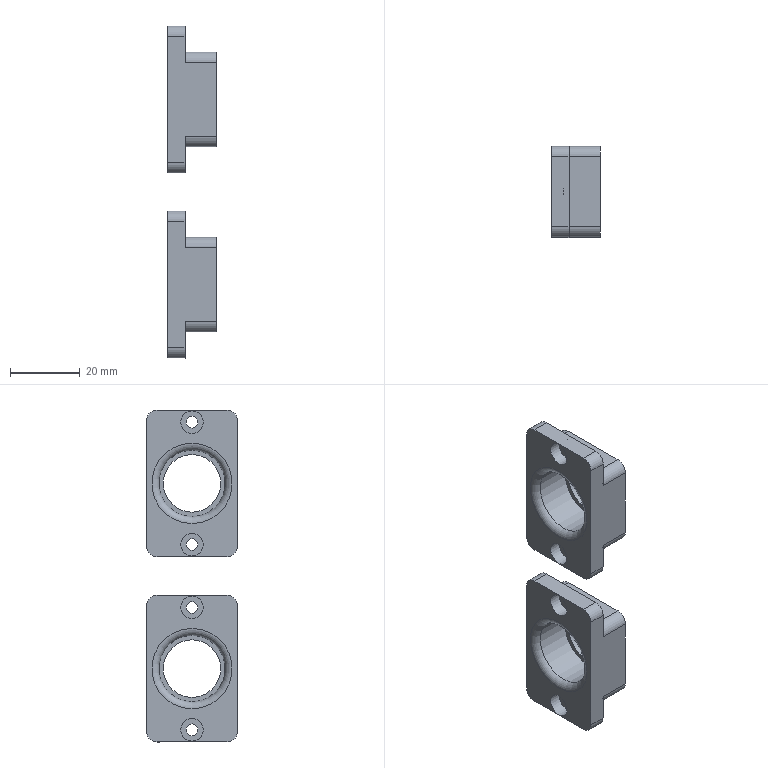CAM job | NX | 3+2 milling, drilling | part box 14 x 26 x 95 mm | stock box 20 x 31 x 100 mm
Tools:
number,name,description,diameter,corner_radius,flute_length,length,flutes
4,D4,平底铣刀-粗,4.0,0.0,25.0,75.0,2
9,D10,平底铣刀-粗,10.0,0.0,35.0,75.0,2
11,D4-J,平底铣刀-精,4.0,0.0,50.0,75.0,2
10,D10-J,平底铣刀-精,10.0,0.0,35.0,75.0,2
18,D6R0.5,圆鼻刀-粗,6.0,0.5,50.0,75.0,2
1,D80R0.8_ENDMILL,圆鼻刀-粗,80.0,0.8,50.0,75.0,2
1,D80R0.8_ENDMILL_J,圆鼻刀-精,80.0,0.8,50.0,75.0,2
2,D6_CHAMFER,倒角刀,6.0,0.0,3.0,25.0,2
13,ZT3.4,钻头,3.4,0.0,35.0,50.0,2
17,ZT12,钻头,12.0,0.0,35.0,50.0,2
Operations:
program,operation,operation_type,tool,method,geometry_group,spindle_rpm,surface_speed,feed_per_tooth,feed_cut,feed_plunge,cut_length_mm,path_length_mm,cut_time_min,machine_time_min
B,FLOOR_WALL_FACE_ROUGH_COPY,VolumeBased25DMillingOperation,D80R0.8_ENDMILL,LAYER_ROUGH_DEPTHK_STEPG,W-B,2800.0,703.696,0.5357,3000.0,100.0,2235.134,4484.512,0.745,0.97
B,FLOOR_WALL_FACE_FINISH_COPY,VolumeBased25DMillingOperation,D80R0.8_ENDMILL_J,SIDE_FINISH_DEPTHK_STEPG,W-B,4000.0,1005.28,0.125,1000.0,100.0,202.998,238.998,0.203,0.2066
B,FLOOR_WALL_LAYER_ROUGH_MID_COPY,VolumeBased25DMillingOperation,D10,LAYER_ROUGH_DEPTHK_STEPG,W-B,8000.0,251.32,0.25,4000.0,100.0,6162.702,6562.022,1.541,1.581
B,DRILL_CHAMFER_1,Operation,D6_CHAMFER,METHOD,W-B,8000.0,150.796,0.0625,1000.0,0.0,20.0,195.505,0.02,0.0376
B,PLANAR_DEBURR_6X45L_COPY,SurfaceContour,D6_CHAMFER,CLIMB_CHAMFER_DEPTH0_STEPG,W-B,6500.0,122.519,0.1154,1500.0,100.0,615.862,1132.723,0.4106,0.4623
B,FLOOR_WALL_SIDE_FINISH_MID_SEL_FLOOR_COPY,VolumeBased25DMillingOperation,D10-J,SIDE_FINISH_DEPTHK_STEPG,W-B,8000.0,251.32,0.0625,1000.0,100.0,213.103,374.652,0.2131,0.2293
A,TOP_FACE,FaceMilling,D80R0.8_ENDMILL,SIDE_FINISH_DEPTHK_STEPG,W-A,4000.0,1005.31,0.125,1000.0,100.0,189.0,225.0,0.189,0.1926
A,PROFILE_ROUGH_2,VolumeBased25DMillingOperation,D10,METHOD,W-A,8000.0,251.327,0.3125,5000.0,80.0,6518.825,6677.325,1.304,1.32
A,CSK_SPOT_DEPTH0.8,Operation,D6_CHAMFER,NONE,W-A,8000.0,150.796,0.0312,500.0,90.0,10.8,154.742,0.0216,0.036
A,CSK_DRILL_SEG0,Operation,ZT3.4,NONE,W-A,2800.0,29.908,0.0179,100.0,90.0,36.086,203.228,0.3609,0.3776
A,CSK_DRILL_SEG0_2,Operation,ZT12,NONE,W-A,800.0,41.469,0.0938,150.0,90.0,41.21,176.43,0.2747,0.2883
A,HOLE_ROUGH_D8_1,CylinderMilling,D10,NONE,W-A,8000.0,201.062,0.075,1200.0,100.0,1465.465,1621.465,1.221,1.237
A,FLOOR_WALL_SPIRAL_ROUGH_MID_COPY,VolumeBased25DMillingOperation,D10,LAYER_ROUGH_DEPTHK_STEPG,W-A,8000.0,251.327,0.125,2000.0,100.0,436.89,619.291,0.2184,0.2367
A,ZLEVEL_SPIRAL_CLIMB_COPY,ZLevelMilling,D10,ZLEVEL_CLIMB_DEPTHK_STEPG,W-A,7000.0,219.911,0.3571,5000.0,100.0,1131.178,1256.293,0.2262,0.2387
A,HOLE_ROUGH_D4_1,CylinderMilling,D4,NONE,W-A,8000.0,100.531,0.075,1200.0,100.0,419.412,714.012,0.3495,0.379
A,HOLE_FINISH_D4_1,CylinderMilling,D4-J,FINISH_STEP_DEPTH_OFF,W-A,8000.0,100.531,0.0312,500.0,100.0,75.825,370.425,0.1516,0.1811
A,ZLEVEL_SPIRAL_CLIMB_COPY_COPY,ZLevelMilling,D6R0.5,ZLEVEL_CLIMB_DEPTHK_STEPG,W-A,7000.0,131.947,0.2857,4000.0,100.0,3737.082,3872.266,0.9343,0.9478
A,SELECTED_BODIES_ONLY,SurfaceContour,D6_CHAMFER,METHOD,W-A,8000.0,150.796,0.1875,3000.0,100.0,296.33,421.431,0.0988,0.1113
A,MILL_CHAMFER_1,PlanarMilling,D6_CHAMFER,NONE,W-A,8000.0,150.796,0.0312,500.0,100.0,117.022,362.762,0.234,0.2586
A,FLOOR_WALL_SIDE_FINISH_MID_COPY,VolumeBased25DMillingOperation,D10-J,SIDE_FINISH_DEPTHK_STEPG,W-A,8000.0,251.32,0.0625,1000.0,100.0,75.181,208.974,0.0752,0.0886
A,FLOOR_WALL_SIDE_FINISH_MID_COPY_1,VolumeBased25DMillingOperation,D10-J,SIDE_FINISH_DEPTHK_STEPG,W-A,8000.0,251.32,0.0625,1000.0,100.0,61.26,207.149,0.0613,0.0758
A,PROFILE_SEMIFINISH_2,VolumeBased25DMillingOperation,D10-J,METHOD,W-A,8000.0,251.327,0.0625,1000.0,100.0,334.559,507.259,0.3346,0.3518